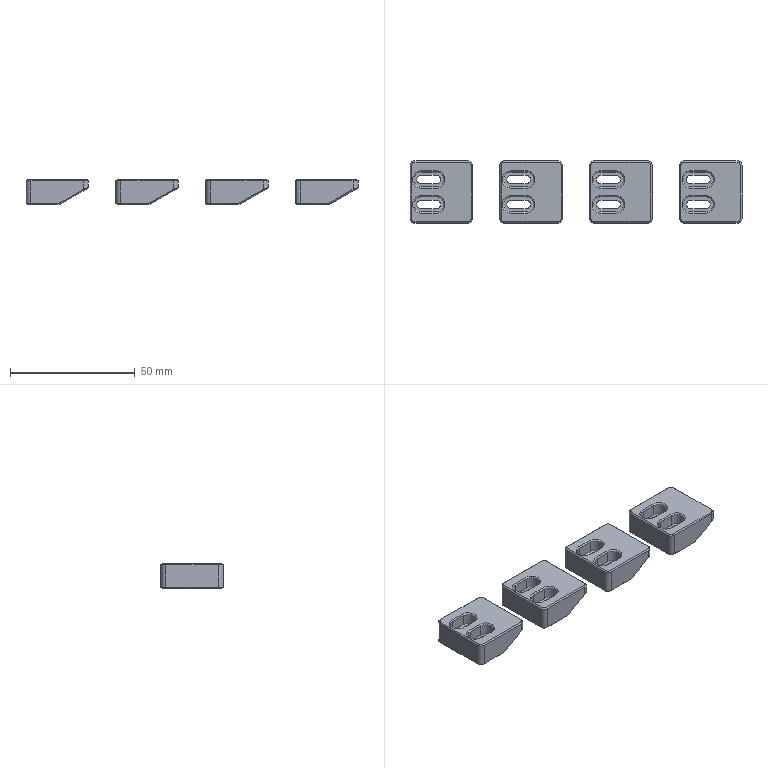NC program | NX | posted with a generic post | part box 133 x 25 x 10 mm
Lines 2353 to 4146 of 9691, first 1540 of 1790 lines:
(ZLEVEL_PROFILE_COPY_1_COPY_COPY_1 , TOOL : D10JING)
N4698 T14 M6
N4700 G54
N4702 G17 G0 G90 X30.145 Y-19.348 S9500 M3
N4704 G43 Z30. H14
N4706 Z-9.
N4708 G94 G1 Z-10. F1000.
N4710 X29.366 Y-18.
N4712 G3 X28.5 Y-17.5 R1.
N4714 G1 X7.5 F1200.
N4716 G2 X0.5 Y-10.5 R7.
N4718 G1 Y10.5
N4720 G2 X7.5 Y17.5 R7.
N4722 G1 X28.5
N4724 G2 X35.5 Y10.5 R7.
N4726 G1 Y-10.5
N4728 G2 X28.5 Y-17.5 R7.
N4730 G3 X27.634 Y-18. R1.
N4732 G1 X26.768 Y-19.5
N4734 Z-9.
N4736 G0 Z30.
N4738 X66.145 Y-19.348
N4740 Z-9.
N4742 G1 Z-10. F1000.
N4744 X65.366 Y-18.
N4746 G3 X64.5 Y-17.5 R1.
N4748 G1 X43.5 F1200.
N4750 G2 X36.5 Y-10.5 R7.
N4752 G1 Y10.5
N4754 G2 X43.5 Y17.5 R7.
N4756 G1 X64.5
N4758 G2 X71.5 Y10.5 R7.
N4760 G1 Y-10.5
N4762 G2 X64.5 Y-17.5 R7.
N4764 G3 X63.634 Y-18. R1.
N4766 G1 X62.768 Y-19.5
N4768 Z-9.
N4770 G0 Z30.
N4772 X-5.855 Y-19.348
N4774 Z-9.
N4776 G1 Z-10. F1000.
N4778 X-6.634 Y-18.
N4780 G3 X-7.5 Y-17.5 R1.
N4782 G1 X-28.5 F1200.
N4784 G2 X-35.5 Y-10.5 R7.
N4786 G1 Y10.5
N4788 G2 X-28.5 Y17.5 R7.
N4790 G1 X-7.5
N4792 G2 X-0.5 Y10.5 R7.
N4794 G1 Y-10.5
N4796 G2 X-7.5 Y-17.5 R7.
N4798 G3 X-8.366 Y-18. R1.
N4800 G1 X-9.232 Y-19.5
N4802 Z-9.
N4804 G0 Z30.
N4806 X-41.855 Y-19.348
N4808 Z-9.
N4810 G1 Z-10. F1000.
N4812 X-42.634 Y-18.
N4814 G3 X-43.5 Y-17.5 R1.
N4816 G1 X-64.5 F1200.
N4818 G2 X-71.5 Y-10.5 R7.
N4820 G1 Y10.5
N4822 G2 X-64.5 Y17.5 R7.
N4824 G1 X-43.5
N4826 G2 X-36.5 Y10.5 R7.
N4828 G1 Y-10.5
N4830 G2 X-43.5 Y-17.5 R7.
N4832 G3 X-44.366 Y-18. R1.
N4834 G1 X-45.232 Y-19.5
N4836 Z-9.
N4838 G0 Z30.
N4840 M5
(ZLEVEL_PROFILE_COPY , TOOL : D3)
N4842 T16 M6
N4844 G54
N4846 G17 G0 G90 X52.179 Y-4.825 S9500 M3
N4848 G43 Z30. H16
N4850 Z1.5
N4852 G94 G1 X52.111 Y-4.75 Z1.495 F1350.
N4854 X45.889 Z1.169
N4856 X45.73 Y-4.926 Z1.156
N4858 X45.851 Y-5.237 Z1.139
N4860 X46. Y-5.25 Z1.131
N4862 X52.023 Y-5.249 Z0.815
N4864 X52.149 Y-5.237 Z0.809
N4866 X52.27 Y-4.926 Z0.791
N4868 X52.111 Y-4.75 Z0.779
N4870 X45.889 Z0.453
N4872 X45.73 Y-4.926 Z0.44
N4874 X45.851 Y-5.237 Z0.423
N4876 X46. Y-5.25 Z0.415
N4878 X52.023 Y-5.249 Z0.099
N4880 X52.149 Y-5.237 Z0.093
N4882 X52.27 Y-4.926 Z0.075
N4884 X52.111 Y-4.75 Z0.063
N4886 X45.889 Z-0.263
N4888 X45.73 Y-4.926 Z-0.276
N4890 X45.851 Y-5.237 Z-0.293
N4892 X45.977 Y-5.249 Z-0.3
N4894 X52.023
N4896 G3 X52. Y-4.75 R0.25
N4898 G1 X46.
N4900 G3 X45.977 Y-5.249 R0.25
N4902 G1 X46.189 Y-5.25 Z-0.306
N4904 X51.914 Z-0.475
N4906 X52.121 Y-5.219 Z-0.481
N4908 X52.244 Y-5.054 Z-0.488
N4910 X52.202 Y-4.853 Z-0.494
N4912 X52.023 Y-4.751 Z-0.5
N4914 X51.811 Y-4.75 Z-0.506
N4916 X48.63 Z-0.6
N4918 X46.
N4920 G3 X45.977 Y-5.249 R0.25
N4922 G1 X46.189 Y-5.25 Z-0.606
N4924 X51.914 Z-0.775
N4926 X52.121 Y-5.219 Z-0.781
N4928 X52.244 Y-5.054 Z-0.788
N4930 X52.202 Y-4.853 Z-0.794
N4932 X52.023 Y-4.751 Z-0.8
N4934 X51.811 Y-4.75 Z-0.806
N4936 X48.63 Z-0.9
N4938 X46.
N4940 G3 X45.977 Y-5.249 R0.25
N4942 G1 X46.189 Y-5.25 Z-0.906
N4944 X51.914 Z-1.075
N4946 X52.121 Y-5.219 Z-1.081
N4948 X52.244 Y-5.054 Z-1.088
N4950 X52.202 Y-4.853 Z-1.094
N4952 X52.023 Y-4.751 Z-1.1
N4954 X51.811 Y-4.75 Z-1.106
N4956 X48.63 Z-1.2
N4958 X46.
N4960 G3 X45.977 Y-5.249 R0.25
N4962 G1 X46.189 Y-5.25 Z-1.206
N4964 X51.914 Z-1.375
N4966 X52.121 Y-5.219 Z-1.381
N4968 X52.244 Y-5.054 Z-1.388
N4970 X52.202 Y-4.853 Z-1.394
N4972 X52.023 Y-4.751 Z-1.4
N4974 X51.811 Y-4.75 Z-1.406
N4976 X48.63 Z-1.5
N4978 X46.
N4980 G3 X45.977 Y-5.249 R0.25
N4982 G1 X46.189 Y-5.25 Z-1.506
N4984 X51.914 Z-1.675
N4986 X52.121 Y-5.219 Z-1.681
N4988 X52.244 Y-5.054 Z-1.688
N4990 X52.202 Y-4.853 Z-1.694
N4992 X52.023 Y-4.751 Z-1.7
N4994 X51.811 Y-4.75 Z-1.706
N4996 X48.63 Z-1.8
N4998 X46.
N5000 G3 X45.977 Y-5.249 R0.25
N5002 G1 X46.189 Y-5.25 Z-1.806
N5004 X51.914 Z-1.975
N5006 X52.121 Y-5.219 Z-1.981
N5008 X52.244 Y-5.054 Z-1.988
N5010 X52.202 Y-4.853 Z-1.994
N5012 X52.023 Y-4.751 Z-2.
N5014 X51.811 Y-4.75 Z-2.006
N5016 X48.63 Z-2.1
N5018 X46.
N5020 G3 X45.977 Y-5.249 R0.25
N5022 G1 X46.189 Y-5.25 Z-2.106
N5024 X51.914 Z-2.275
N5026 X52.121 Y-5.219 Z-2.281
N5028 X52.244 Y-5.054 Z-2.288
N5030 X52.202 Y-4.853 Z-2.294
N5032 X52.023 Y-4.751 Z-2.3
N5034 X51.811 Y-4.75 Z-2.306
N5036 X48.63 Z-2.4
N5038 X46.
N5040 G3 X45.977 Y-5.249 R0.25
N5042 G1 X46.189 Y-5.25 Z-2.406
N5044 X51.914 Z-2.575
N5046 X52.121 Y-5.219 Z-2.581
N5048 X52.244 Y-5.054 Z-2.588
N5050 X52.202 Y-4.853 Z-2.594
N5052 X52.023 Y-4.751 Z-2.6
N5054 X51.811 Y-4.75 Z-2.606
N5056 X48.63 Z-2.7
N5058 X46.
N5060 G3 X45.977 Y-5.249 R0.25
N5062 G1 X46.189 Y-5.25 Z-2.706
N5064 X51.914 Z-2.875
N5066 X52.121 Y-5.219 Z-2.881
N5068 X52.244 Y-5.054 Z-2.888
N5070 X52.202 Y-4.853 Z-2.894
N5072 X52.023 Y-4.751 Z-2.9
N5074 X51.811 Y-4.75 Z-2.906
N5076 X48.63 Z-3.
N5078 X46.
N5080 G3 X45.977 Y-5.249 R0.25
N5082 G1 X46.189 Y-5.25 Z-3.006
N5084 X51.914 Z-3.175
N5086 X52.121 Y-5.219 Z-3.181
N5088 X52.244 Y-5.054 Z-3.188
N5090 X52.202 Y-4.853 Z-3.194
N5092 X52.023 Y-4.751 Z-3.2
N5094 X51.811 Y-4.75 Z-3.206
N5096 X48.63 Z-3.3
N5098 X46.
N5100 G3 X45.977 Y-5.249 R0.25
N5102 G1 X46.189 Y-5.25 Z-3.306
N5104 X51.914 Z-3.475
N5106 X52.121 Y-5.219 Z-3.481
N5108 X52.244 Y-5.054 Z-3.488
N5110 X52.202 Y-4.853 Z-3.494
N5112 X52.023 Y-4.751 Z-3.5
N5114 X51.811 Y-4.75 Z-3.506
N5116 X48.63 Z-3.6
N5118 X46.
N5120 G3 X45.977 Y-5.249 R0.25
N5122 G1 X46.189 Y-5.25 Z-3.606
N5124 X51.914 Z-3.775
N5126 X52.121 Y-5.219 Z-3.781
N5128 X52.244 Y-5.054 Z-3.788
N5130 X52.202 Y-4.853 Z-3.794
N5132 X52.023 Y-4.751 Z-3.8
N5134 X51.811 Y-4.75 Z-3.806
N5136 X48.63 Z-3.9
N5138 X46.
N5140 G3 X45.977 Y-5.249 R0.25
N5142 G1 X46.189 Y-5.25 Z-3.906
N5144 X51.914 Z-4.075
N5146 X52.121 Y-5.219 Z-4.081
N5148 X52.244 Y-5.054 Z-4.088
N5150 X52.202 Y-4.853 Z-4.094
N5152 X52.023 Y-4.751 Z-4.1
N5154 X51.811 Y-4.75 Z-4.106
N5156 X48.63 Z-4.2
N5158 X46.
N5160 G3 X45.977 Y-5.249 R0.25
N5162 G1 X46.189 Y-5.25 Z-4.206
N5164 X51.914 Z-4.375
N5166 X52.121 Y-5.219 Z-4.381
N5168 X52.244 Y-5.054 Z-4.388
N5170 X52.202 Y-4.853 Z-4.394
N5172 X52.023 Y-4.751 Z-4.4
N5174 X51.811 Y-4.75 Z-4.406
N5176 X48.63 Z-4.5
N5178 X46.
N5180 G3 X45.977 Y-5.249 R0.25
N5182 G1 X46.189 Y-5.25 Z-4.505
N5184 X51.914 Z-4.646
N5186 X52.121 Y-5.219 Z-4.651
N5188 X52.244 Y-5.054 Z-4.656
N5190 X52.202 Y-4.853 Z-4.661
N5192 X52.023 Y-4.751 Z-4.667
N5194 X51.811 Y-4.75 Z-4.672
N5196 X48.63 Z-4.75
N5198 X46.
N5200 G3 X45.977 Y-5.249 R0.25
N5202 G1 X46.189 Y-5.25 Z-4.755
N5204 X51.914 Z-4.896
N5206 X52.121 Y-5.219 Z-4.901
N5208 X52.244 Y-5.054 Z-4.906
N5210 X52.202 Y-4.853 Z-4.911
N5212 X52.023 Y-4.751 Z-4.917
N5214 X51.811 Y-4.75 Z-4.922
N5216 X48.63 Z-5.
N5218 X46.
N5220 G3 X45.977 Y-5.249 R0.25
N5222 G1 X46.189 Y-5.25 Z-5.005
N5224 X51.914 Z-5.146
N5226 X52.121 Y-5.219 Z-5.151
N5228 X52.244 Y-5.054 Z-5.156
N5230 X52.202 Y-4.853 Z-5.161
N5232 X52.023 Y-4.751 Z-5.167
N5234 X51.811 Y-4.75 Z-5.172
N5236 X48.63 Z-5.25
N5238 X46.
N5240 G3 X45.977 Y-5.249 R0.25
N5242 G1 X46.189 Y-5.25 Z-5.255
N5244 X51.914 Z-5.396
N5246 X52.121 Y-5.219 Z-5.401
N5248 X52.244 Y-5.054 Z-5.406
N5250 X52.202 Y-4.853 Z-5.411
N5252 X52.023 Y-4.751 Z-5.417
N5254 X51.811 Y-4.75 Z-5.422
N5256 X48.63 Z-5.5
N5258 X46.
N5260 G3 X45.75 Y-5. R0.25
N5262 X46. Y-5.25 R0.25
N5264 G1 X52.
N5266 G3 X52.25 Y-5. R0.25
N5268 X52. Y-4.75 R0.25
N5270 G1 X48.63
N5272 Z-4.
N5274 G0 Z30.
N5276 X45.821 Y4.825
N5278 Z1.5
N5280 G1 X45.889 Y4.75 Z1.495
N5282 X52.111 Z1.169
N5284 X52.27 Y4.926 Z1.156
N5286 X52.149 Y5.237 Z1.139
N5288 X52. Y5.25 Z1.131
N5290 X45.977 Y5.249 Z0.815
N5292 X45.851 Y5.237 Z0.809
N5294 X45.73 Y4.926 Z0.791
N5296 X45.889 Y4.75 Z0.779
N5298 X52.111 Z0.453
N5300 X52.27 Y4.926 Z0.44
N5302 X52.149 Y5.237 Z0.423
N5304 X52. Y5.25 Z0.415
N5306 X45.977 Y5.249 Z0.099
N5308 X45.851 Y5.237 Z0.093
N5310 X45.73 Y4.926 Z0.075
N5312 X45.889 Y4.75 Z0.063
N5314 X52.111 Z-0.263
N5316 X52.27 Y4.926 Z-0.276
N5318 X52.149 Y5.237 Z-0.293
N5320 X52.023 Y5.249 Z-0.3
N5322 X45.977
N5324 G3 X46. Y4.75 R0.25
N5326 G1 X52.
N5328 G3 X52.023 Y5.249 R0.25
N5330 G1 X51.811 Y5.25 Z-0.306
N5332 X46.086 Z-0.475
N5334 X45.879 Y5.219 Z-0.481
N5336 X45.756 Y5.054 Z-0.488
N5338 X45.798 Y4.853 Z-0.494
N5340 X45.977 Y4.751 Z-0.5
N5342 X46.189 Y4.75 Z-0.506
N5344 X49.37 Z-0.6
N5346 X52.
N5348 G3 X52.023 Y5.249 R0.25
N5350 G1 X51.811 Y5.25 Z-0.606
N5352 X46.086 Z-0.775
N5354 X45.879 Y5.219 Z-0.781
N5356 X45.756 Y5.054 Z-0.788
N5358 X45.798 Y4.853 Z-0.794
N5360 X45.977 Y4.751 Z-0.8
N5362 X46.189 Y4.75 Z-0.806
N5364 X49.37 Z-0.9
N5366 X52.
N5368 G3 X52.023 Y5.249 R0.25
N5370 G1 X51.811 Y5.25 Z-0.906
N5372 X46.086 Z-1.075
N5374 X45.879 Y5.219 Z-1.081
N5376 X45.756 Y5.054 Z-1.088
N5378 X45.798 Y4.853 Z-1.094
N5380 X45.977 Y4.751 Z-1.1
N5382 X46.189 Y4.75 Z-1.106
N5384 X49.37 Z-1.2
N5386 X52.
N5388 G3 X52.023 Y5.249 R0.25
N5390 G1 X51.811 Y5.25 Z-1.206
N5392 X46.086 Z-1.375
N5394 X45.879 Y5.219 Z-1.381
N5396 X45.756 Y5.054 Z-1.388
N5398 X45.798 Y4.853 Z-1.394
N5400 X45.977 Y4.751 Z-1.4
N5402 X46.189 Y4.75 Z-1.406
N5404 X49.37 Z-1.5
N5406 X52.
N5408 G3 X52.023 Y5.249 R0.25
N5410 G1 X51.811 Y5.25 Z-1.506
N5412 X46.086 Z-1.675
N5414 X45.879 Y5.219 Z-1.681
N5416 X45.756 Y5.054 Z-1.688
N5418 X45.798 Y4.853 Z-1.694
N5420 X45.977 Y4.751 Z-1.7
N5422 X46.189 Y4.75 Z-1.706
N5424 X49.37 Z-1.8
N5426 X52.
N5428 G3 X52.023 Y5.249 R0.25
N5430 G1 X51.811 Y5.25 Z-1.806
N5432 X46.086 Z-1.975
N5434 X45.879 Y5.219 Z-1.981
N5436 X45.756 Y5.054 Z-1.988
N5438 X45.798 Y4.853 Z-1.994
N5440 X45.977 Y4.751 Z-2.
N5442 X46.189 Y4.75 Z-2.006
N5444 X49.37 Z-2.1
N5446 X52.
N5448 G3 X52.023 Y5.249 R0.25
N5450 G1 X51.811 Y5.25 Z-2.106
N5452 X46.086 Z-2.275
N5454 X45.879 Y5.219 Z-2.281
N5456 X45.756 Y5.054 Z-2.288
N5458 X45.798 Y4.853 Z-2.294
N5460 X45.977 Y4.751 Z-2.3
N5462 X46.189 Y4.75 Z-2.306
N5464 X49.37 Z-2.4
N5466 X52.
N5468 G3 X52.023 Y5.249 R0.25
N5470 G1 X51.811 Y5.25 Z-2.406
N5472 X46.086 Z-2.575
N5474 X45.879 Y5.219 Z-2.581
N5476 X45.756 Y5.054 Z-2.588
N5478 X45.798 Y4.853 Z-2.594
N5480 X45.977 Y4.751 Z-2.6
N5482 X46.189 Y4.75 Z-2.606
N5484 X49.37 Z-2.7
N5486 X52.
N5488 G3 X52.023 Y5.249 R0.25
N5490 G1 X51.811 Y5.25 Z-2.706
N5492 X46.086 Z-2.875
N5494 X45.879 Y5.219 Z-2.881
N5496 X45.756 Y5.054 Z-2.888
N5498 X45.798 Y4.853 Z-2.894
N5500 X45.977 Y4.751 Z-2.9
N5502 X46.189 Y4.75 Z-2.906
N5504 X49.37 Z-3.
N5506 X52.
N5508 G3 X52.023 Y5.249 R0.25
N5510 G1 X51.811 Y5.25 Z-3.006
N5512 X46.086 Z-3.175
N5514 X45.879 Y5.219 Z-3.181
N5516 X45.756 Y5.054 Z-3.188
N5518 X45.798 Y4.853 Z-3.194
N5520 X45.977 Y4.751 Z-3.2
N5522 X46.189 Y4.75 Z-3.206
N5524 X49.37 Z-3.3
N5526 X52.
N5528 G3 X52.023 Y5.249 R0.25
N5530 G1 X51.811 Y5.25 Z-3.306
N5532 X46.086 Z-3.475
N5534 X45.879 Y5.219 Z-3.481
N5536 X45.756 Y5.054 Z-3.488
N5538 X45.798 Y4.853 Z-3.494
N5540 X45.977 Y4.751 Z-3.5
N5542 X46.189 Y4.75 Z-3.506
N5544 X49.37 Z-3.6
N5546 X52.
N5548 G3 X52.023 Y5.249 R0.25
N5550 G1 X51.811 Y5.25 Z-3.606
N5552 X46.086 Z-3.775
N5554 X45.879 Y5.219 Z-3.781
N5556 X45.756 Y5.054 Z-3.788
N5558 X45.798 Y4.853 Z-3.794
N5560 X45.977 Y4.751 Z-3.8
N5562 X46.189 Y4.75 Z-3.806
N5564 X49.37 Z-3.9
N5566 X52.
N5568 G3 X52.023 Y5.249 R0.25
N5570 G1 X51.811 Y5.25 Z-3.906
N5572 X46.086 Z-4.075
N5574 X45.879 Y5.219 Z-4.081
N5576 X45.756 Y5.054 Z-4.088
N5578 X45.798 Y4.853 Z-4.094
N5580 X45.977 Y4.751 Z-4.1
N5582 X46.189 Y4.75 Z-4.106
N5584 X49.37 Z-4.2
N5586 X52.
N5588 G3 X52.023 Y5.249 R0.25
N5590 G1 X51.811 Y5.25 Z-4.206
N5592 X46.086 Z-4.375
N5594 X45.879 Y5.219 Z-4.381
N5596 X45.756 Y5.054 Z-4.388
N5598 X45.798 Y4.853 Z-4.394
N5600 X45.977 Y4.751 Z-4.4
N5602 X46.189 Y4.75 Z-4.406
N5604 X49.37 Z-4.5
N5606 X52.
N5608 G3 X52.023 Y5.249 R0.25
N5610 G1 X51.811 Y5.25 Z-4.505
N5612 X46.086 Z-4.646
N5614 X45.879 Y5.219 Z-4.651
N5616 X45.756 Y5.054 Z-4.656
N5618 X45.798 Y4.853 Z-4.661
N5620 X45.977 Y4.751 Z-4.667
N5622 X46.189 Y4.75 Z-4.672
N5624 X49.37 Z-4.75
N5626 X52.
N5628 G3 X52.023 Y5.249 R0.25
N5630 G1 X51.811 Y5.25 Z-4.755
N5632 X46.086 Z-4.896
N5634 X45.879 Y5.219 Z-4.901
N5636 X45.756 Y5.054 Z-4.906
N5638 X45.798 Y4.853 Z-4.911
N5640 X45.977 Y4.751 Z-4.917
N5642 X46.189 Y4.75 Z-4.922
N5644 X49.37 Z-5.
N5646 X52.
N5648 G3 X52.023 Y5.249 R0.25
N5650 G1 X51.811 Y5.25 Z-5.005
N5652 X46.086 Z-5.146
N5654 X45.879 Y5.219 Z-5.151
N5656 X45.756 Y5.054 Z-5.156
N5658 X45.798 Y4.853 Z-5.161
N5660 X45.977 Y4.751 Z-5.167
N5662 X46.189 Y4.75 Z-5.172
N5664 X49.37 Z-5.25
N5666 X52.
N5668 G3 X52.023 Y5.249 R0.25
N5670 G1 X51.811 Y5.25 Z-5.255
N5672 X46.086 Z-5.396
N5674 X45.879 Y5.219 Z-5.401
N5676 X45.756 Y5.054 Z-5.406
N5678 X45.798 Y4.853 Z-5.411
N5680 X45.977 Y4.751 Z-5.417
N5682 X46.189 Y4.75 Z-5.422
N5684 X49.37 Z-5.5
N5686 X52.
N5688 G3 X52.25 Y5. R0.25
N5690 X52. Y5.25 R0.25
N5692 G1 X46.
N5694 G3 X45.75 Y5. R0.25
N5696 X46. Y4.75 R0.25
N5698 G1 X49.37
N5700 Z-4.
N5702 G0 Z30.
N5704 X16.179 Y-4.825
N5706 Z1.5
N5708 G1 X16.111 Y-4.75 Z1.495
N5710 X9.889 Z1.169
N5712 X9.73 Y-4.926 Z1.156
N5714 X9.851 Y-5.237 Z1.139
N5716 X10. Y-5.25 Z1.131
N5718 X16.023 Y-5.249 Z0.815
N5720 X16.149 Y-5.237 Z0.809
N5722 X16.27 Y-4.926 Z0.791
N5724 X16.111 Y-4.75 Z0.779
N5726 X9.889 Z0.453
N5728 X9.73 Y-4.926 Z0.44
N5730 X9.851 Y-5.237 Z0.423
N5732 X10. Y-5.25 Z0.415
N5734 X16.023 Y-5.249 Z0.099
N5736 X16.149 Y-5.237 Z0.093
N5738 X16.27 Y-4.926 Z0.075
N5740 X16.111 Y-4.75 Z0.063
N5742 X9.889 Z-0.263
N5744 X9.73 Y-4.926 Z-0.276
N5746 X9.851 Y-5.237 Z-0.293
N5748 X9.977 Y-5.249 Z-0.3
N5750 X16.023
N5752 G3 X16. Y-4.75 R0.25
N5754 G1 X10.
N5756 G3 X9.977 Y-5.249 R0.25
N5758 G1 X10.189 Y-5.25 Z-0.306
N5760 X15.914 Z-0.475
N5762 X16.121 Y-5.219 Z-0.481
N5764 X16.244 Y-5.054 Z-0.488
N5766 X16.202 Y-4.853 Z-0.494
N5768 X16.023 Y-4.751 Z-0.5
N5770 X15.811 Y-4.75 Z-0.506
N5772 X12.63 Z-0.6
N5774 X10.
N5776 G3 X9.977 Y-5.249 R0.25
N5778 G1 X10.189 Y-5.25 Z-0.606
N5780 X15.914 Z-0.775
N5782 X16.121 Y-5.219 Z-0.781
N5784 X16.244 Y-5.054 Z-0.788
N5786 X16.202 Y-4.853 Z-0.794
N5788 X16.023 Y-4.751 Z-0.8
N5790 X15.811 Y-4.75 Z-0.806
N5792 X12.63 Z-0.9
N5794 X10.
N5796 G3 X9.977 Y-5.249 R0.25
N5798 G1 X10.189 Y-5.25 Z-0.906
N5800 X15.914 Z-1.075
N5802 X16.121 Y-5.219 Z-1.081
N5804 X16.244 Y-5.054 Z-1.088
N5806 X16.202 Y-4.853 Z-1.094
N5808 X16.023 Y-4.751 Z-1.1
N5810 X15.811 Y-4.75 Z-1.106
N5812 X12.63 Z-1.2
N5814 X10.
N5816 G3 X9.977 Y-5.249 R0.25
N5818 G1 X10.189 Y-5.25 Z-1.206
N5820 X15.914 Z-1.375
N5822 X16.121 Y-5.219 Z-1.381
N5824 X16.244 Y-5.054 Z-1.388
N5826 X16.202 Y-4.853 Z-1.394
N5828 X16.023 Y-4.751 Z-1.4
N5830 X15.811 Y-4.75 Z-1.406
N5832 X12.63 Z-1.5
N5834 X10.
N5836 G3 X9.977 Y-5.249 R0.25
N5838 G1 X10.189 Y-5.25 Z-1.506
N5840 X15.914 Z-1.675
N5842 X16.121 Y-5.219 Z-1.681
N5844 X16.244 Y-5.054 Z-1.688
N5846 X16.202 Y-4.853 Z-1.694
N5848 X16.023 Y-4.751 Z-1.7
N5850 X15.811 Y-4.75 Z-1.706
N5852 X12.63 Z-1.8
N5854 X10.
N5856 G3 X9.977 Y-5.249 R0.25
N5858 G1 X10.189 Y-5.25 Z-1.806
N5860 X15.914 Z-1.975
N5862 X16.121 Y-5.219 Z-1.981
N5864 X16.244 Y-5.054 Z-1.988
N5866 X16.202 Y-4.853 Z-1.994
N5868 X16.023 Y-4.751 Z-2.
N5870 X15.811 Y-4.75 Z-2.006
N5872 X12.63 Z-2.1
N5874 X10.
N5876 G3 X9.977 Y-5.249 R0.25
N5878 G1 X10.189 Y-5.25 Z-2.106
N5880 X15.914 Z-2.275
N5882 X16.121 Y-5.219 Z-2.281
N5884 X16.244 Y-5.054 Z-2.288
N5886 X16.202 Y-4.853 Z-2.294
N5888 X16.023 Y-4.751 Z-2.3
N5890 X15.811 Y-4.75 Z-2.306
N5892 X12.63 Z-2.4
N5894 X10.
N5896 G3 X9.977 Y-5.249 R0.25
N5898 G1 X10.189 Y-5.25 Z-2.406
N5900 X15.914 Z-2.575
N5902 X16.121 Y-5.219 Z-2.581
N5904 X16.244 Y-5.054 Z-2.588
N5906 X16.202 Y-4.853 Z-2.594
N5908 X16.023 Y-4.751 Z-2.6
N5910 X15.811 Y-4.75 Z-2.606
N5912 X12.63 Z-2.7
N5914 X10.
N5916 G3 X9.977 Y-5.249 R0.25
N5918 G1 X10.189 Y-5.25 Z-2.706
N5920 X15.914 Z-2.875
N5922 X16.121 Y-5.219 Z-2.881
N5924 X16.244 Y-5.054 Z-2.888
N5926 X16.202 Y-4.853 Z-2.894
N5928 X16.023 Y-4.751 Z-2.9
N5930 X15.811 Y-4.75 Z-2.906
N5932 X12.63 Z-3.
N5934 X10.
N5936 G3 X9.977 Y-5.249 R0.25
N5938 G1 X10.189 Y-5.25 Z-3.006
N5940 X15.914 Z-3.175
N5942 X16.121 Y-5.219 Z-3.181
N5944 X16.244 Y-5.054 Z-3.188
N5946 X16.202 Y-4.853 Z-3.194
N5948 X16.023 Y-4.751 Z-3.2
N5950 X15.811 Y-4.75 Z-3.206
N5952 X12.63 Z-3.3
N5954 X10.
N5956 G3 X9.977 Y-5.249 R0.25
N5958 G1 X10.189 Y-5.25 Z-3.306
N5960 X15.914 Z-3.475
N5962 X16.121 Y-5.219 Z-3.481
N5964 X16.244 Y-5.054 Z-3.488
N5966 X16.202 Y-4.853 Z-3.494
N5968 X16.023 Y-4.751 Z-3.5
N5970 X15.811 Y-4.75 Z-3.506
N5972 X12.63 Z-3.6
N5974 X10.
N5976 G3 X9.977 Y-5.249 R0.25
N5978 G1 X10.189 Y-5.25 Z-3.606
N5980 X15.914 Z-3.775
N5982 X16.121 Y-5.219 Z-3.781
N5984 X16.244 Y-5.054 Z-3.788
N5986 X16.202 Y-4.853 Z-3.794
N5988 X16.023 Y-4.751 Z-3.8
N5990 X15.811 Y-4.75 Z-3.806
N5992 X12.63 Z-3.9
N5994 X10.
N5996 G3 X9.977 Y-5.249 R0.25
N5998 G1 X10.189 Y-5.25 Z-3.906
N6000 X15.914 Z-4.075
N6002 X16.121 Y-5.219 Z-4.081
N6004 X16.244 Y-5.054 Z-4.088
N6006 X16.202 Y-4.853 Z-4.094
N6008 X16.023 Y-4.751 Z-4.1
N6010 X15.811 Y-4.75 Z-4.106
N6012 X12.63 Z-4.2
N6014 X10.
N6016 G3 X9.977 Y-5.249 R0.25
N6018 G1 X10.189 Y-5.25 Z-4.206
N6020 X15.914 Z-4.375
N6022 X16.121 Y-5.219 Z-4.381
N6024 X16.244 Y-5.054 Z-4.388
N6026 X16.202 Y-4.853 Z-4.394
N6028 X16.023 Y-4.751 Z-4.4
N6030 X15.811 Y-4.75 Z-4.406
N6032 X12.63 Z-4.5
N6034 X10.
N6036 G3 X9.977 Y-5.249 R0.25
N6038 G1 X10.189 Y-5.25 Z-4.505
N6040 X15.914 Z-4.646
N6042 X16.121 Y-5.219 Z-4.651
N6044 X16.244 Y-5.054 Z-4.656
N6046 X16.202 Y-4.853 Z-4.661
N6048 X16.023 Y-4.751 Z-4.667
N6050 X15.811 Y-4.75 Z-4.672
N6052 X12.63 Z-4.75
N6054 X10.
N6056 G3 X9.977 Y-5.249 R0.25
N6058 G1 X10.189 Y-5.25 Z-4.755
N6060 X15.914 Z-4.896
N6062 X16.121 Y-5.219 Z-4.901
N6064 X16.244 Y-5.054 Z-4.906
N6066 X16.202 Y-4.853 Z-4.911
N6068 X16.023 Y-4.751 Z-4.917
N6070 X15.811 Y-4.75 Z-4.922
N6072 X12.63 Z-5.
N6074 X10.
N6076 G3 X9.977 Y-5.249 R0.25
N6078 G1 X10.189 Y-5.25 Z-5.005
N6080 X15.914 Z-5.146
N6082 X16.121 Y-5.219 Z-5.151
N6084 X16.244 Y-5.054 Z-5.156
N6086 X16.202 Y-4.853 Z-5.161
N6088 X16.023 Y-4.751 Z-5.167
N6090 X15.811 Y-4.75 Z-5.172
N6092 X12.63 Z-5.25
N6094 X10.
N6096 G3 X9.977 Y-5.249 R0.25
N6098 G1 X10.189 Y-5.25 Z-5.255
N6100 X15.914 Z-5.396
N6102 X16.121 Y-5.219 Z-5.401
N6104 X16.244 Y-5.054 Z-5.406
N6106 X16.202 Y-4.853 Z-5.411
N6108 X16.023 Y-4.751 Z-5.417
N6110 X15.811 Y-4.75 Z-5.422
N6112 X12.63 Z-5.5
N6114 X10.
N6116 G3 X9.75 Y-5. R0.25
N6118 X10. Y-5.25 R0.25
N6120 G1 X16.
N6122 G3 X16.25 Y-5. R0.25
N6124 X16. Y-4.75 R0.25
N6126 G1 X12.63
N6128 Z-4.
N6130 G0 Z30.
N6132 X9.821 Y4.825
N6134 Z1.5
N6136 G1 X9.889 Y4.75 Z1.495
N6138 X16.111 Z1.169
N6140 X16.27 Y4.926 Z1.156
N6142 X16.149 Y5.237 Z1.139
N6144 X16. Y5.25 Z1.131
N6146 X9.977 Y5.249 Z0.815
N6148 X9.851 Y5.237 Z0.809
N6150 X9.73 Y4.926 Z0.791
N6152 X9.889 Y4.75 Z0.779
N6154 X16.111 Z0.453
N6156 X16.27 Y4.926 Z0.44
N6158 X16.149 Y5.237 Z0.423
N6160 X16. Y5.25 Z0.415
N6162 X9.977 Y5.249 Z0.099
N6164 X9.851 Y5.237 Z0.093
N6166 X9.73 Y4.926 Z0.075
N6168 X9.889 Y4.75 Z0.063
N6170 X16.111 Z-0.263
N6172 X16.27 Y4.926 Z-0.276
N6174 X16.149 Y5.237 Z-0.293
N6176 X16.023 Y5.249 Z-0.3
N6178 X9.977
N6180 G3 X10. Y4.75 R0.25
N6182 G1 X16.
N6184 G3 X16.023 Y5.249 R0.25
N6186 G1 X15.811 Y5.25 Z-0.306
N6188 X10.086 Z-0.475
N6190 X9.879 Y5.219 Z-0.481
N6192 X9.756 Y5.054 Z-0.488
N6194 X9.798 Y4.853 Z-0.494
N6196 X9.977 Y4.751 Z-0.5
N6198 X10.189 Y4.75 Z-0.506
N6200 X13.37 Z-0.6
N6202 X16.
N6204 G3 X16.023 Y5.249 R0.25
N6206 G1 X15.811 Y5.25 Z-0.606
N6208 X10.086 Z-0.775
N6210 X9.879 Y5.219 Z-0.781
N6212 X9.756 Y5.054 Z-0.788
N6214 X9.798 Y4.853 Z-0.794
N6216 X9.977 Y4.751 Z-0.8
N6218 X10.189 Y4.75 Z-0.806
N6220 X13.37 Z-0.9
N6222 X16.
N6224 G3 X16.023 Y5.249 R0.25
N6226 G1 X15.811 Y5.25 Z-0.906
N6228 X10.086 Z-1.075
N6230 X9.879 Y5.219 Z-1.081
N6232 X9.756 Y5.054 Z-1.088
N6234 X9.798 Y4.853 Z-1.094
N6236 X9.977 Y4.751 Z-1.1
N6238 X10.189 Y4.75 Z-1.106
N6240 X13.37 Z-1.2
N6242 X16.
N6244 G3 X16.023 Y5.249 R0.25
N6246 G1 X15.811 Y5.25 Z-1.206
N6248 X10.086 Z-1.375
N6250 X9.879 Y5.219 Z-1.381
N6252 X9.756 Y5.054 Z-1.388
N6254 X9.798 Y4.853 Z-1.394
N6256 X9.977 Y4.751 Z-1.4
N6258 X10.189 Y4.75 Z-1.406
N6260 X13.37 Z-1.5
N6262 X16.
N6264 G3 X16.023 Y5.249 R0.25
N6266 G1 X15.811 Y5.25 Z-1.506
N6268 X10.086 Z-1.675
N6270 X9.879 Y5.219 Z-1.681
N6272 X9.756 Y5.054 Z-1.688
N6274 X9.798 Y4.853 Z-1.694
N6276 X9.977 Y4.751 Z-1.7
N6278 X10.189 Y4.75 Z-1.706
N6280 X13.37 Z-1.8
N6282 X16.
N6284 G3 X16.023 Y5.249 R0.25
N6286 G1 X15.811 Y5.25 Z-1.806
N6288 X10.086 Z-1.975
N6290 X9.879 Y5.219 Z-1.981
N6292 X9.756 Y5.054 Z-1.988
N6294 X9.798 Y4.853 Z-1.994
N6296 X9.977 Y4.751 Z-2.
N6298 X10.189 Y4.75 Z-2.006
N6300 X13.37 Z-2.1
N6302 X16.
N6304 G3 X16.023 Y5.249 R0.25
N6306 G1 X15.811 Y5.25 Z-2.106
N6308 X10.086 Z-2.275
N6310 X9.879 Y5.219 Z-2.281
N6312 X9.756 Y5.054 Z-2.288
N6314 X9.798 Y4.853 Z-2.294
N6316 X9.977 Y4.751 Z-2.3
N6318 X10.189 Y4.75 Z-2.306
N6320 X13.37 Z-2.4
N6322 X16.
N6324 G3 X16.023 Y5.249 R0.25
N6326 G1 X15.811 Y5.25 Z-2.406
N6328 X10.086 Z-2.575
N6330 X9.879 Y5.219 Z-2.581
N6332 X9.756 Y5.054 Z-2.588
N6334 X9.798 Y4.853 Z-2.594
N6336 X9.977 Y4.751 Z-2.6
N6338 X10.189 Y4.75 Z-2.606
N6340 X13.37 Z-2.7
N6342 X16.
N6344 G3 X16.023 Y5.249 R0.25
N6346 G1 X15.811 Y5.25 Z-2.706
N6348 X10.086 Z-2.875
N6350 X9.879 Y5.219 Z-2.881
N6352 X9.756 Y5.054 Z-2.888
N6354 X9.798 Y4.853 Z-2.894
N6356 X9.977 Y4.751 Z-2.9
N6358 X10.189 Y4.75 Z-2.906
N6360 X13.37 Z-3.
N6362 X16.
N6364 G3 X16.023 Y5.249 R0.25
N6366 G1 X15.811 Y5.25 Z-3.006
N6368 X10.086 Z-3.175
N6370 X9.879 Y5.219 Z-3.181
N6372 X9.756 Y5.054 Z-3.188
N6374 X9.798 Y4.853 Z-3.194
N6376 X9.977 Y4.751 Z-3.2
N6378 X10.189 Y4.75 Z-3.206
N6380 X13.37 Z-3.3
N6382 X16.
N6384 G3 X16.023 Y5.249 R0.25
N6386 G1 X15.811 Y5.25 Z-3.306
N6388 X10.086 Z-3.475
N6390 X9.879 Y5.219 Z-3.481
N6392 X9.756 Y5.054 Z-3.488
N6394 X9.798 Y4.853 Z-3.494
N6396 X9.977 Y4.751 Z-3.5
N6398 X10.189 Y4.75 Z-3.506
N6400 X13.37 Z-3.6
N6402 X16.
N6404 G3 X16.023 Y5.249 R0.25
N6406 G1 X15.811 Y5.25 Z-3.606
N6408 X10.086 Z-3.775
N6410 X9.879 Y5.219 Z-3.781
N6412 X9.756 Y5.054 Z-3.788
N6414 X9.798 Y4.853 Z-3.794
N6416 X9.977 Y4.751 Z-3.8
N6418 X10.189 Y4.75 Z-3.806
N6420 X13.37 Z-3.9
N6422 X16.
N6424 G3 X16.023 Y5.249 R0.25
N6426 G1 X15.811 Y5.25 Z-3.906
N6428 X10.086 Z-4.075
N6430 X9.879 Y5.219 Z-4.081
N6432 X9.756 Y5.054 Z-4.088
N6434 X9.798 Y4.853 Z-4.094
N6436 X9.977 Y4.751 Z-4.1
N6438 X10.189 Y4.75 Z-4.106
N6440 X13.37 Z-4.2
N6442 X16.
N6444 G3 X16.023 Y5.249 R0.25
N6446 G1 X15.811 Y5.25 Z-4.206
N6448 X10.086 Z-4.375
N6450 X9.879 Y5.219 Z-4.381
N6452 X9.756 Y5.054 Z-4.388
N6454 X9.798 Y4.853 Z-4.394
N6456 X9.977 Y4.751 Z-4.4
N6458 X10.189 Y4.75 Z-4.406
N6460 X13.37 Z-4.5
N6462 X16.
N6464 G3 X16.023 Y5.249 R0.25
N6466 G1 X15.811 Y5.25 Z-4.505
N6468 X10.086 Z-4.646
N6470 X9.879 Y5.219 Z-4.651
N6472 X9.756 Y5.054 Z-4.656
N6474 X9.798 Y4.853 Z-4.661
N6476 X9.977 Y4.751 Z-4.667
N6478 X10.189 Y4.75 Z-4.672
N6480 X13.37 Z-4.75
N6482 X16.
N6484 G3 X16.023 Y5.249 R0.25
N6486 G1 X15.811 Y5.25 Z-4.755
N6488 X10.086 Z-4.896
N6490 X9.879 Y5.219 Z-4.901
N6492 X9.756 Y5.054 Z-4.906
N6494 X9.798 Y4.853 Z-4.911
N6496 X9.977 Y4.751 Z-4.917
N6498 X10.189 Y4.75 Z-4.922
N6500 X13.37 Z-5.
N6502 X16.
N6504 G3 X16.023 Y5.249 R0.25
N6506 G1 X15.811 Y5.25 Z-5.005
N6508 X10.086 Z-5.146
N6510 X9.879 Y5.219 Z-5.151
N6512 X9.756 Y5.054 Z-5.156
N6514 X9.798 Y4.853 Z-5.161
N6516 X9.977 Y4.751 Z-5.167
N6518 X10.189 Y4.75 Z-5.172
N6520 X13.37 Z-5.25
N6522 X16.
N6524 G3 X16.023 Y5.249 R0.25
N6526 G1 X15.811 Y5.25 Z-5.255
N6528 X10.086 Z-5.396
N6530 X9.879 Y5.219 Z-5.401
N6532 X9.756 Y5.054 Z-5.406
N6534 X9.798 Y4.853 Z-5.411
N6536 X9.977 Y4.751 Z-5.417
N6538 X10.189 Y4.75 Z-5.422
N6540 X13.37 Z-5.5
N6542 X16.
N6544 G3 X16.25 Y5. R0.25
N6546 X16. Y5.25 R0.25
N6548 G1 X10.
N6550 G3 X9.75 Y5. R0.25
N6552 X10. Y4.75 R0.25
N6554 G1 X13.37
N6556 Z-4.
N6558 G0 Z30.
N6560 X-19.821 Y-4.825
N6562 Z1.5
N6564 G1 X-19.889 Y-4.75 Z1.495
N6566 X-26.111 Z1.169
N6568 X-26.27 Y-4.926 Z1.156
N6570 X-26.149 Y-5.237 Z1.139
N6572 X-26. Y-5.25 Z1.131
N6574 X-19.977 Y-5.249 Z0.815
N6576 X-19.851 Y-5.237 Z0.809
N6578 X-19.73 Y-4.926 Z0.791
N6580 X-19.889 Y-4.75 Z0.779
N6582 X-26.111 Z0.453
N6584 X-26.27 Y-4.926 Z0.44
N6586 X-26.149 Y-5.237 Z0.423
N6588 X-26. Y-5.25 Z0.415
N6590 X-19.977 Y-5.249 Z0.099
N6592 X-19.851 Y-5.237 Z0.093
N6594 X-19.73 Y-4.926 Z0.075
N6596 X-19.889 Y-4.75 Z0.063
N6598 X-26.111 Z-0.263
N6600 X-26.27 Y-4.926 Z-0.276
N6602 X-26.149 Y-5.237 Z-0.293
N6604 X-26.023 Y-5.249 Z-0.3
N6606 X-19.977
N6608 G3 X-20. Y-4.75 R0.25
N6610 G1 X-26.
N6612 G3 X-26.023 Y-5.249 R0.25
N6614 G1 X-25.811 Y-5.25 Z-0.306
N6616 X-20.086 Z-0.475
N6618 X-19.879 Y-5.219 Z-0.481
N6620 X-19.756 Y-5.054 Z-0.488
N6622 X-19.798 Y-4.853 Z-0.494
N6624 X-19.977 Y-4.751 Z-0.5
N6626 X-20.189 Y-4.75 Z-0.506
N6628 X-23.37 Z-0.6
N6630 X-26.
N6632 G3 X-26.023 Y-5.249 R0.25
N6634 G1 X-25.811 Y-5.25 Z-0.606
N6636 X-20.086 Z-0.775
N6638 X-19.879 Y-5.219 Z-0.781
N6640 X-19.756 Y-5.054 Z-0.788
N6642 X-19.798 Y-4.853 Z-0.794
N6644 X-19.977 Y-4.751 Z-0.8
N6646 X-20.189 Y-4.75 Z-0.806
N6648 X-23.37 Z-0.9
N6650 X-26.
N6652 G3 X-26.023 Y-5.249 R0.25
N6654 G1 X-25.811 Y-5.25 Z-0.906
N6656 X-20.086 Z-1.075
N6658 X-19.879 Y-5.219 Z-1.081
N6660 X-19.756 Y-5.054 Z-1.088
N6662 X-19.798 Y-4.853 Z-1.094
N6664 X-19.977 Y-4.751 Z-1.1
N6666 X-20.189 Y-4.75 Z-1.106
N6668 X-23.37 Z-1.2
N6670 X-26.
N6672 G3 X-26.023 Y-5.249 R0.25
N6674 G1 X-25.811 Y-5.25 Z-1.206
N6676 X-20.086 Z-1.375
N6678 X-19.879 Y-5.219 Z-1.381
N6680 X-19.756 Y-5.054 Z-1.388
N6682 X-19.798 Y-4.853 Z-1.394
N6684 X-19.977 Y-4.751 Z-1.4
N6686 X-20.189 Y-4.75 Z-1.406
N6688 X-23.37 Z-1.5
N6690 X-26.
N6692 G3 X-26.023 Y-5.249 R0.25
N6694 G1 X-25.811 Y-5.25 Z-1.506
N6696 X-20.086 Z-1.675
N6698 X-19.879 Y-5.219 Z-1.681
N6700 X-19.756 Y-5.054 Z-1.688
N6702 X-19.798 Y-4.853 Z-1.694
N6704 X-19.977 Y-4.751 Z-1.7
N6706 X-20.189 Y-4.75 Z-1.706
N6708 X-23.37 Z-1.8
N6710 X-26.
N6712 G3 X-26.023 Y-5.249 R0.25
N6714 G1 X-25.811 Y-5.25 Z-1.806
N6716 X-20.086 Z-1.975
N6718 X-19.879 Y-5.219 Z-1.981
N6720 X-19.756 Y-5.054 Z-1.988
N6722 X-19.798 Y-4.853 Z-1.994
N6724 X-19.977 Y-4.751 Z-2.
N6726 X-20.189 Y-4.75 Z-2.006
N6728 X-23.37 Z-2.1
N6730 X-26.
N6732 G3 X-26.023 Y-5.249 R0.25
N6734 G1 X-25.811 Y-5.25 Z-2.106
N6736 X-20.086 Z-2.275
N6738 X-19.879 Y-5.219 Z-2.281
N6740 X-19.756 Y-5.054 Z-2.288
N6742 X-19.798 Y-4.853 Z-2.294
N6744 X-19.977 Y-4.751 Z-2.3
N6746 X-20.189 Y-4.75 Z-2.306
N6748 X-23.37 Z-2.4
N6750 X-26.
N6752 G3 X-26.023 Y-5.249 R0.25
N6754 G1 X-25.811 Y-5.25 Z-2.406
N6756 X-20.086 Z-2.575
N6758 X-19.879 Y-5.219 Z-2.581
N6760 X-19.756 Y-5.054 Z-2.588
N6762 X-19.798 Y-4.853 Z-2.594
N6764 X-19.977 Y-4.751 Z-2.6
N6766 X-20.189 Y-4.75 Z-2.606
N6768 X-23.37 Z-2.7
N6770 X-26.
N6772 G3 X-26.023 Y-5.249 R0.25
N6774 G1 X-25.811 Y-5.25 Z-2.706
N6776 X-20.086 Z-2.875
N6778 X-19.879 Y-5.219 Z-2.881
N6780 X-19.756 Y-5.054 Z-2.888
N6782 X-19.798 Y-4.853 Z-2.894
N6784 X-19.977 Y-4.751 Z-2.9
N6786 X-20.189 Y-4.75 Z-2.906
N6788 X-23.37 Z-3.
N6790 X-26.
N6792 G3 X-26.023 Y-5.249 R0.25
N6794 G1 X-25.811 Y-5.25 Z-3.006
N6796 X-20.086 Z-3.175
N6798 X-19.879 Y-5.219 Z-3.181
N6800 X-19.756 Y-5.054 Z-3.188
N6802 X-19.798 Y-4.853 Z-3.194
N6804 X-19.977 Y-4.751 Z-3.2
N6806 X-20.189 Y-4.75 Z-3.206
N6808 X-23.37 Z-3.3
N6810 X-26.
N6812 G3 X-26.023 Y-5.249 R0.25
N6814 G1 X-25.811 Y-5.25 Z-3.306
N6816 X-20.086 Z-3.475
N6818 X-19.879 Y-5.219 Z-3.481
N6820 X-19.756 Y-5.054 Z-3.488
N6822 X-19.798 Y-4.853 Z-3.494
N6824 X-19.977 Y-4.751 Z-3.5
N6826 X-20.189 Y-4.75 Z-3.506
N6828 X-23.37 Z-3.6
N6830 X-26.
N6832 G3 X-26.023 Y-5.249 R0.25
N6834 G1 X-25.811 Y-5.25 Z-3.606
N6836 X-20.086 Z-3.775
N6838 X-19.879 Y-5.219 Z-3.781
N6840 X-19.756 Y-5.054 Z-3.788
N6842 X-19.798 Y-4.853 Z-3.794
N6844 X-19.977 Y-4.751 Z-3.8
N6846 X-20.189 Y-4.75 Z-3.806
N6848 X-23.37 Z-3.9
N6850 X-26.
N6852 G3 X-26.023 Y-5.249 R0.25
N6854 G1 X-25.811 Y-5.25 Z-3.906
N6856 X-20.086 Z-4.075
N6858 X-19.879 Y-5.219 Z-4.081
N6860 X-19.756 Y-5.054 Z-4.088
N6862 X-19.798 Y-4.853 Z-4.094
N6864 X-19.977 Y-4.751 Z-4.1
N6866 X-20.189 Y-4.75 Z-4.106
N6868 X-23.37 Z-4.2
N6870 X-26.
N6872 G3 X-26.023 Y-5.249 R0.25
N6874 G1 X-25.811 Y-5.25 Z-4.206
N6876 X-20.086 Z-4.375
N6878 X-19.879 Y-5.219 Z-4.381
N6880 X-19.756 Y-5.054 Z-4.388
N6882 X-19.798 Y-4.853 Z-4.394
N6884 X-19.977 Y-4.751 Z-4.4
N6886 X-20.189 Y-4.75 Z-4.406
N6888 X-23.37 Z-4.5
N6890 X-26.
N6892 G3 X-26.023 Y-5.249 R0.25
N6894 G1 X-25.811 Y-5.25 Z-4.505
N6896 X-20.086 Z-4.646
N6898 X-19.879 Y-5.219 Z-4.651
N6900 X-19.756 Y-5.054 Z-4.656
N6902 X-19.798 Y-4.853 Z-4.661
N6904 X-19.977 Y-4.751 Z-4.667
N6906 X-20.189 Y-4.75 Z-4.672
N6908 X-23.37 Z-4.75
N6910 X-26.
N6912 G3 X-26.023 Y-5.249 R0.25
N6914 G1 X-25.811 Y-5.25 Z-4.755
N6916 X-20.086 Z-4.896
N6918 X-19.879 Y-5.219 Z-4.901
N6920 X-19.756 Y-5.054 Z-4.906
N6922 X-19.798 Y-4.853 Z-4.911
N6924 X-19.977 Y-4.751 Z-4.917
N6926 X-20.189 Y-4.75 Z-4.922
N6928 X-23.37 Z-5.
N6930 X-26.
N6932 G3 X-26.023 Y-5.249 R0.25
N6934 G1 X-25.811 Y-5.25 Z-5.005
N6936 X-20.086 Z-5.146
N6938 X-19.879 Y-5.219 Z-5.151
N6940 X-19.756 Y-5.054 Z-5.156
N6942 X-19.798 Y-4.853 Z-5.161
N6944 X-19.977 Y-4.751 Z-5.167
N6946 X-20.189 Y-4.75 Z-5.172
N6948 X-23.37 Z-5.25
N6950 X-26.
N6952 G3 X-26.023 Y-5.249 R0.25
N6954 G1 X-25.811 Y-5.25 Z-5.255
N6956 X-20.086 Z-5.396
N6958 X-19.879 Y-5.219 Z-5.401
N6960 X-19.756 Y-5.054 Z-5.406
N6962 X-19.798 Y-4.853 Z-5.411
N6964 X-19.977 Y-4.751 Z-5.417
N6966 X-20.189 Y-4.75 Z-5.422
N6968 X-23.37 Z-5.5
N6970 X-26.
N6972 G3 X-26.25 Y-5. R0.25
N6974 X-26. Y-5.25 R0.25
N6976 G1 X-20.
N6978 G3 X-19.75 Y-5. R0.25
N6980 X-20. Y-4.75 R0.25
N6982 G1 X-23.37
N6984 Z-4.
N6986 G0 Z30.
N6988 X-26.179 Y4.825
N6990 Z1.5
N6992 G1 X-26.111 Y4.75 Z1.495
N6994 X-19.889 Z1.169
N6996 X-19.73 Y4.926 Z1.156
N6998 X-19.851 Y5.237 Z1.139
N7000 X-20. Y5.25 Z1.131
N7002 X-26.023 Y5.249 Z0.815
N7004 X-26.149 Y5.237 Z0.809
N7006 X-26.27 Y4.926 Z0.791
N7008 X-26.111 Y4.75 Z0.779
N7010 X-19.889 Z0.453
N7012 X-19.73 Y4.926 Z0.44
N7014 X-19.851 Y5.237 Z0.423
N7016 X-20. Y5.25 Z0.415
N7018 X-26.023 Y5.249 Z0.099
N7020 X-26.149 Y5.237 Z0.093
N7022 X-26.27 Y4.926 Z0.075
N7024 X-26.111 Y4.75 Z0.063
N7026 X-19.889 Z-0.263
N7028 X-19.73 Y4.926 Z-0.276
N7030 X-19.851 Y5.237 Z-0.293
N7032 X-19.977 Y5.249 Z-0.3
N7034 X-26.023
N7036 G3 X-26. Y4.75 R0.25
N7038 G1 X-20.
N7040 G3 X-19.977 Y5.249 R0.25
N7042 G1 X-20.189 Y5.25 Z-0.306
N7044 X-25.914 Z-0.475
N7046 X-26.121 Y5.219 Z-0.481
N7048 X-26.244 Y5.054 Z-0.488
N7050 X-26.202 Y4.853 Z-0.494
N7052 X-26.023 Y4.751 Z-0.5
N7054 X-25.811 Y4.75 Z-0.506
N7056 X-22.63 Z-0.6
N7058 X-20.
N7060 G3 X-19.977 Y5.249 R0.25
N7062 G1 X-20.189 Y5.25 Z-0.606
N7064 X-25.914 Z-0.775
N7066 X-26.121 Y5.219 Z-0.781
N7068 X-26.244 Y5.054 Z-0.788
N7070 X-26.202 Y4.853 Z-0.794
N7072 X-26.023 Y4.751 Z-0.8
N7074 X-25.811 Y4.75 Z-0.806
N7076 X-22.63 Z-0.9
N7078 X-20.
N7080 G3 X-19.977 Y5.249 R0.25
N7082 G1 X-20.189 Y5.25 Z-0.906
N7084 X-25.914 Z-1.075
N7086 X-26.121 Y5.219 Z-1.081
N7088 X-26.244 Y5.054 Z-1.088
N7090 X-26.202 Y4.853 Z-1.094
N7092 X-26.023 Y4.751 Z-1.1
N7094 X-25.811 Y4.75 Z-1.106
N7096 X-22.63 Z-1.2
N7098 X-20.
N7100 G3 X-19.977 Y5.249 R0.25
N7102 G1 X-20.189 Y5.25 Z-1.206
N7104 X-25.914 Z-1.375
N7106 X-26.121 Y5.219 Z-1.381
N7108 X-26.244 Y5.054 Z-1.388
N7110 X-26.202 Y4.853 Z-1.394
N7112 X-26.023 Y4.751 Z-1.4
N7114 X-25.811 Y4.75 Z-1.406
N7116 X-22.63 Z-1.5
N7118 X-20.
N7120 G3 X-19.977 Y5.249 R0.25
N7122 G1 X-20.189 Y5.25 Z-1.506
N7124 X-25.914 Z-1.675
N7126 X-26.121 Y5.219 Z-1.681
N7128 X-26.244 Y5.054 Z-1.688
N7130 X-26.202 Y4.853 Z-1.694
N7132 X-26.023 Y4.751 Z-1.7
N7134 X-25.811 Y4.75 Z-1.706
N7136 X-22.63 Z-1.8
N7138 X-20.
N7140 G3 X-19.977 Y5.249 R0.25
N7142 G1 X-20.189 Y5.25 Z-1.806
N7144 X-25.914 Z-1.975
N7146 X-26.121 Y5.219 Z-1.981
N7148 X-26.244 Y5.054 Z-1.988
N7150 X-26.202 Y4.853 Z-1.994
N7152 X-26.023 Y4.751 Z-2.
N7154 X-25.811 Y4.75 Z-2.006
N7156 X-22.63 Z-2.1
N7158 X-20.
N7160 G3 X-19.977 Y5.249 R0.25
N7162 G1 X-20.189 Y5.25 Z-2.106
N7164 X-25.914 Z-2.275
N7166 X-26.121 Y5.219 Z-2.281
N7168 X-26.244 Y5.054 Z-2.288
N7170 X-26.202 Y4.853 Z-2.294
N7172 X-26.023 Y4.751 Z-2.3
N7174 X-25.811 Y4.75 Z-2.306
N7176 X-22.63 Z-2.4
N7178 X-20.
N7180 G3 X-19.977 Y5.249 R0.25
N7182 G1 X-20.189 Y5.25 Z-2.406
N7184 X-25.914 Z-2.575
N7186 X-26.121 Y5.219 Z-2.581
N7188 X-26.244 Y5.054 Z-2.588
N7190 X-26.202 Y4.853 Z-2.594
N7192 X-26.023 Y4.751 Z-2.6
N7194 X-25.811 Y4.75 Z-2.606
N7196 X-22.63 Z-2.7
N7198 X-20.
N7200 G3 X-19.977 Y5.249 R0.25
N7202 G1 X-20.189 Y5.25 Z-2.706
N7204 X-25.914 Z-2.875
N7206 X-26.121 Y5.219 Z-2.881
N7208 X-26.244 Y5.054 Z-2.888
N7210 X-26.202 Y4.853 Z-2.894
N7212 X-26.023 Y4.751 Z-2.9
N7214 X-25.811 Y4.75 Z-2.906
N7216 X-22.63 Z-3.
N7218 X-20.
N7220 G3 X-19.977 Y5.249 R0.25
N7222 G1 X-20.189 Y5.25 Z-3.006
N7224 X-25.914 Z-3.175
N7226 X-26.121 Y5.219 Z-3.181
N7228 X-26.244 Y5.054 Z-3.188
N7230 X-26.202 Y4.853 Z-3.194
N7232 X-26.023 Y4.751 Z-3.2
N7234 X-25.811 Y4.75 Z-3.206
N7236 X-22.63 Z-3.3
N7238 X-20.
N7240 G3 X-19.977 Y5.249 R0.25
N7242 G1 X-20.189 Y5.25 Z-3.306
N7244 X-25.914 Z-3.475
N7246 X-26.121 Y5.219 Z-3.481
N7248 X-26.244 Y5.054 Z-3.488
N7250 X-26.202 Y4.853 Z-3.494
N7252 X-26.023 Y4.751 Z-3.5
N7254 X-25.811 Y4.75 Z-3.506
N7256 X-22.63 Z-3.6
N7258 X-20.
N7260 G3 X-19.977 Y5.249 R0.25
N7262 G1 X-20.189 Y5.25 Z-3.606
N7264 X-25.914 Z-3.775
N7266 X-26.121 Y5.219 Z-3.781
N7268 X-26.244 Y5.054 Z-3.788
N7270 X-26.202 Y4.853 Z-3.794
N7272 X-26.023 Y4.751 Z-3.8
N7274 X-25.811 Y4.75 Z-3.806
N7276 X-22.63 Z-3.9
N7278 X-20.
N7280 G3 X-19.977 Y5.249 R0.25
N7282 G1 X-20.189 Y5.25 Z-3.906
N7284 X-25.914 Z-4.075
N7286 X-26.121 Y5.219 Z-4.081
N7288 X-26.244 Y5.054 Z-4.088
N7290 X-26.202 Y4.853 Z-4.094
N7292 X-26.023 Y4.751 Z-4.1
N7294 X-25.811 Y4.75 Z-4.106
N7296 X-22.63 Z-4.2
N7298 X-20.
N7300 G3 X-19.977 Y5.249 R0.25
N7302 G1 X-20.189 Y5.25 Z-4.206
N7304 X-25.914 Z-4.375
N7306 X-26.121 Y5.219 Z-4.381
N7308 X-26.244 Y5.054 Z-4.388
N7310 X-26.202 Y4.853 Z-4.394
N7312 X-26.023 Y4.751 Z-4.4
N7314 X-25.811 Y4.75 Z-4.406
N7316 X-22.63 Z-4.5
N7318 X-20.
N7320 G3 X-19.977 Y5.249 R0.25
N7322 G1 X-20.189 Y5.25 Z-4.505
N7324 X-25.914 Z-4.646
N7326 X-26.121 Y5.219 Z-4.651
N7328 X-26.244 Y5.054 Z-4.656
N7330 X-26.202 Y4.853 Z-4.661
N7332 X-26.023 Y4.751 Z-4.667
N7334 X-25.811 Y4.75 Z-4.672
N7336 X-22.63 Z-4.75
N7338 X-20.
N7340 G3 X-19.977 Y5.249 R0.25
N7342 G1 X-20.189 Y5.25 Z-4.755
N7344 X-25.914 Z-4.896
N7346 X-26.121 Y5.219 Z-4.901
N7348 X-26.244 Y5.054 Z-4.906
N7350 X-26.202 Y4.853 Z-4.911
N7352 X-26.023 Y4.751 Z-4.917
N7354 X-25.811 Y4.75 Z-4.922
N7356 X-22.63 Z-5.
N7358 X-20.
N7360 G3 X-19.977 Y5.249 R0.25
N7362 G1 X-20.189 Y5.25 Z-5.005
N7364 X-25.914 Z-5.146
N7366 X-26.121 Y5.219 Z-5.151
N7368 X-26.244 Y5.054 Z-5.156
N7370 X-26.202 Y4.853 Z-5.161
N7372 X-26.023 Y4.751 Z-5.167
N7374 X-25.811 Y4.75 Z-5.172
N7376 X-22.63 Z-5.25
N7378 X-20.
N7380 G3 X-19.977 Y5.249 R0.25
N7382 G1 X-20.189 Y5.25 Z-5.255
N7384 X-25.914 Z-5.396
N7386 X-26.121 Y5.219 Z-5.401
N7388 X-26.244 Y5.054 Z-5.406
N7390 X-26.202 Y4.853 Z-5.411
N7392 X-26.023 Y4.751 Z-5.417
N7394 X-25.811 Y4.75 Z-5.422
N7396 X-22.63 Z-5.5
N7398 X-20.
N7400 G3 X-19.75 Y5. R0.25
N7402 X-20. Y5.25 R0.25
N7404 G1 X-26.
N7406 G3 X-26.25 Y5. R0.25
N7408 X-26. Y4.75 R0.25
N7410 G1 X-22.63
N7412 Z-4.
N7414 G0 Z30.
N7416 X-55.821 Y-4.825
N7418 Z1.5
N7420 G1 X-55.889 Y-4.75 Z1.495
N7422 X-62.111 Z1.169
N7424 X-62.27 Y-4.926 Z1.156
N7426 X-62.149 Y-5.237 Z1.139
N7428 X-62. Y-5.25 Z1.131
N7430 X-55.977 Y-5.249 Z0.815
N7432 X-55.851 Y-5.237 Z0.809
N7434 X-55.73 Y-4.926 Z0.791
N7436 X-55.889 Y-4.75 Z0.779
N7438 X-62.111 Z0.453
N7440 X-62.27 Y-4.926 Z0.44
N7442 X-62.149 Y-5.237 Z0.423
N7444 X-62. Y-5.25 Z0.415
N7446 X-55.977 Y-5.249 Z0.099
N7448 X-55.851 Y-5.237 Z0.093
N7450 X-55.73 Y-4.926 Z0.075
N7452 X-55.889 Y-4.75 Z0.063
N7454 X-62.111 Z-0.263
N7456 X-62.27 Y-4.926 Z-0.276
N7458 X-62.149 Y-5.237 Z-0.293
N7460 X-62.023 Y-5.249 Z-0.3
N7462 X-55.977
N7464 G3 X-56. Y-4.75 R0.25
N7466 G1 X-62.
N7468 G3 X-62.023 Y-5.249 R0.25
N7470 G1 X-61.811 Y-5.25 Z-0.306
N7472 X-56.086 Z-0.475
N7474 X-55.879 Y-5.219 Z-0.481
N7476 X-55.756 Y-5.054 Z-0.488
N7478 X-55.798 Y-4.853 Z-0.494
N7480 X-55.977 Y-4.751 Z-0.5
N7482 X-56.189 Y-4.75 Z-0.506
N7484 X-59.37 Z-0.6
N7486 X-62.
N7488 G3 X-62.023 Y-5.249 R0.25
N7490 G1 X-61.811 Y-5.25 Z-0.606
N7492 X-56.086 Z-0.775
N7494 X-55.879 Y-5.219 Z-0.781
N7496 X-55.756 Y-5.054 Z-0.788
N7498 X-55.798 Y-4.853 Z-0.794
N7500 X-55.977 Y-4.751 Z-0.8
N7502 X-56.189 Y-4.75 Z-0.806
N7504 X-59.37 Z-0.9
N7506 X-62.
N7508 G3 X-62.023 Y-5.249 R0.25
N7510 G1 X-61.811 Y-5.25 Z-0.906
N7512 X-56.086 Z-1.075
N7514 X-55.879 Y-5.219 Z-1.081
N7516 X-55.756 Y-5.054 Z-1.088
N7518 X-55.798 Y-4.853 Z-1.094
N7520 X-55.977 Y-4.751 Z-1.1
N7522 X-56.189 Y-4.75 Z-1.106
N7524 X-59.37 Z-1.2
N7526 X-62.
N7528 G3 X-62.023 Y-5.249 R0.25
N7530 G1 X-61.811 Y-5.25 Z-1.206
N7532 X-56.086 Z-1.375
N7534 X-55.879 Y-5.219 Z-1.381
N7536 X-55.756 Y-5.054 Z-1.388
N7538 X-55.798 Y-4.853 Z-1.394
N7540 X-55.977 Y-4.751 Z-1.4
N7542 X-56.189 Y-4.75 Z-1.406
N7544 X-59.37 Z-1.5
N7546 X-62.
N7548 G3 X-62.023 Y-5.249 R0.25
N7550 G1 X-61.811 Y-5.25 Z-1.506
N7552 X-56.086 Z-1.675
N7554 X-55.879 Y-5.219 Z-1.681
N7556 X-55.756 Y-5.054 Z-1.688
N7558 X-55.798 Y-4.853 Z-1.694
N7560 X-55.977 Y-4.751 Z-1.7
N7562 X-56.189 Y-4.75 Z-1.706
N7564 X-59.37 Z-1.8
N7566 X-62.
N7568 G3 X-62.023 Y-5.249 R0.25
N7570 G1 X-61.811 Y-5.25 Z-1.806
N7572 X-56.086 Z-1.975
N7574 X-55.879 Y-5.219 Z-1.981
N7576 X-55.756 Y-5.054 Z-1.988
N7578 X-55.798 Y-4.853 Z-1.994
N7580 X-55.977 Y-4.751 Z-2.
N7582 X-56.189 Y-4.75 Z-2.006
N7584 X-59.37 Z-2.1
N7586 X-62.
N7588 G3 X-62.023 Y-5.249 R0.25
N7590 G1 X-61.811 Y-5.25 Z-2.106
N7592 X-56.086 Z-2.275
N7594 X-55.879 Y-5.219 Z-2.281
N7596 X-55.756 Y-5.054 Z-2.288
N7598 X-55.798 Y-4.853 Z-2.294
N7600 X-55.977 Y-4.751 Z-2.3
N7602 X-56.189 Y-4.75 Z-2.306
N7604 X-59.37 Z-2.4
N7606 X-62.
N7608 G3 X-62.023 Y-5.249 R0.25
N7610 G1 X-61.811 Y-5.25 Z-2.406
N7612 X-56.086 Z-2.575
N7614 X-55.879 Y-5.219 Z-2.581
N7616 X-55.756 Y-5.054 Z-2.588
N7618 X-55.798 Y-4.853 Z-2.594
N7620 X-55.977 Y-4.751 Z-2.6
N7622 X-56.189 Y-4.75 Z-2.606
N7624 X-59.37 Z-2.7
N7626 X-62.
N7628 G3 X-62.023 Y-5.249 R0.25
N7630 G1 X-61.811 Y-5.25 Z-2.706
N7632 X-56.086 Z-2.875
N7634 X-55.879 Y-5.219 Z-2.881
N7636 X-55.756 Y-5.054 Z-2.888
N7638 X-55.798 Y-4.853 Z-2.894
N7640 X-55.977 Y-4.751 Z-2.9
N7642 X-56.189 Y-4.75 Z-2.906
N7644 X-59.37 Z-3.
N7646 X-62.
N7648 G3 X-62.023 Y-5.249 R0.25
N7650 G1 X-61.811 Y-5.25 Z-3.006
N7652 X-56.086 Z-3.175
N7654 X-55.879 Y-5.219 Z-3.181
N7656 X-55.756 Y-5.054 Z-3.188
N7658 X-55.798 Y-4.853 Z-3.194
N7660 X-55.977 Y-4.751 Z-3.2
N7662 X-56.189 Y-4.75 Z-3.206
N7664 X-59.37 Z-3.3
N7666 X-62.
N7668 G3 X-62.023 Y-5.249 R0.25
N7670 G1 X-61.811 Y-5.25 Z-3.306
N7672 X-56.086 Z-3.475
N7674 X-55.879 Y-5.219 Z-3.481
N7676 X-55.756 Y-5.054 Z-3.488
N7678 X-55.798 Y-4.853 Z-3.494
N7680 X-55.977 Y-4.751 Z-3.5
N7682 X-56.189 Y-4.75 Z-3.506
N7684 X-59.37 Z-3.6
N7686 X-62.
N7688 G3 X-62.023 Y-5.249 R0.25
N7690 G1 X-61.811 Y-5.25 Z-3.606
N7692 X-56.086 Z-3.775
N7694 X-55.879 Y-5.219 Z-3.781
N7696 X-55.756 Y-5.054 Z-3.788
N7698 X-55.798 Y-4.853 Z-3.794
N7700 X-55.977 Y-4.751 Z-3.8
N7702 X-56.189 Y-4.75 Z-3.806
N7704 X-59.37 Z-3.9
N7706 X-62.
N7708 G3 X-62.023 Y-5.249 R0.25
N7710 G1 X-61.811 Y-5.25 Z-3.906
N7712 X-56.086 Z-4.075
N7714 X-55.879 Y-5.219 Z-4.081
N7716 X-55.756 Y-5.054 Z-4.088
N7718 X-55.798 Y-4.853 Z-4.094
N7720 X-55.977 Y-4.751 Z-4.1
N7722 X-56.189 Y-4.75 Z-4.106
N7724 X-59.37 Z-4.2
N7726 X-62.
N7728 G3 X-62.023 Y-5.249 R0.25
N7730 G1 X-61.811 Y-5.25 Z-4.206
N7732 X-56.086 Z-4.375
N7734 X-55.879 Y-5.219 Z-4.381
N7736 X-55.756 Y-5.054 Z-4.388
N7738 X-55.798 Y-4.853 Z-4.394
N7740 X-55.977 Y-4.751 Z-4.4
N7742 X-56.189 Y-4.75 Z-4.406
N7744 X-59.37 Z-4.5
N7746 X-62.
N7748 G3 X-62.023 Y-5.249 R0.25
N7750 G1 X-61.811 Y-5.25 Z-4.505
N7752 X-56.086 Z-4.646
N7754 X-55.879 Y-5.219 Z-4.651
N7756 X-55.756 Y-5.054 Z-4.656
N7758 X-55.798 Y-4.853 Z-4.661
N7760 X-55.977 Y-4.751 Z-4.667
N7762 X-56.189 Y-4.75 Z-4.672
N7764 X-59.37 Z-4.75
N7766 X-62.
N7768 G3 X-62.023 Y-5.249 R0.25
N7770 G1 X-61.811 Y-5.25 Z-4.755
N7772 X-56.086 Z-4.896